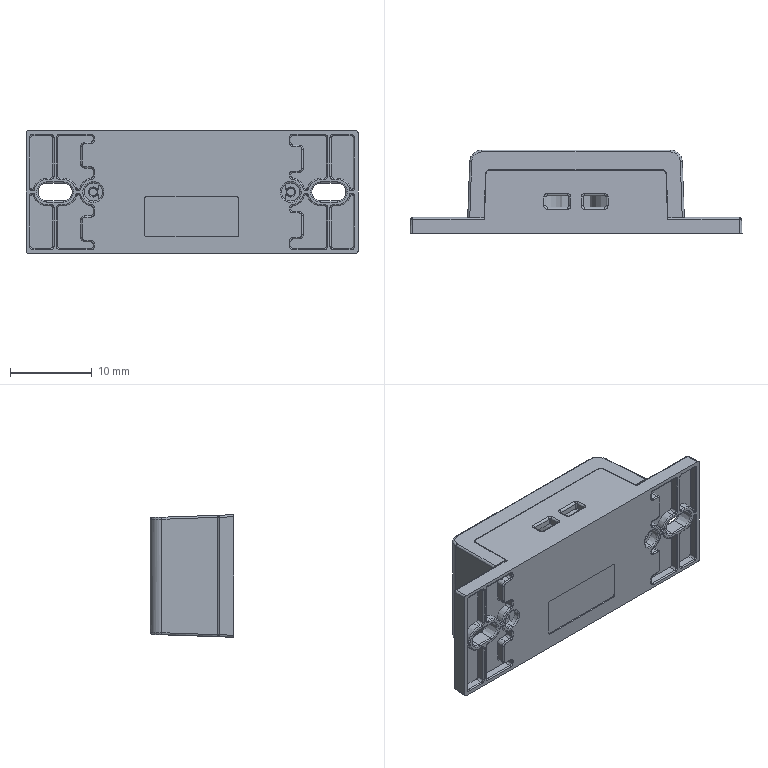Part | SolidWorks | features BaseBody 3, CombineBodies 1, MoveFace 1, Scale 1 | 1 solid | 676 faces | box 40.625 x 10.25 x 15 mm | volume 2277 mm3 | plane 262 | cylinder 184 | spline 140 | cone 90 | commonest cylinder face diameters 0.3 x96 0.5 x42 1 x16 1.25 x6 2.25 x6 0.95 x4